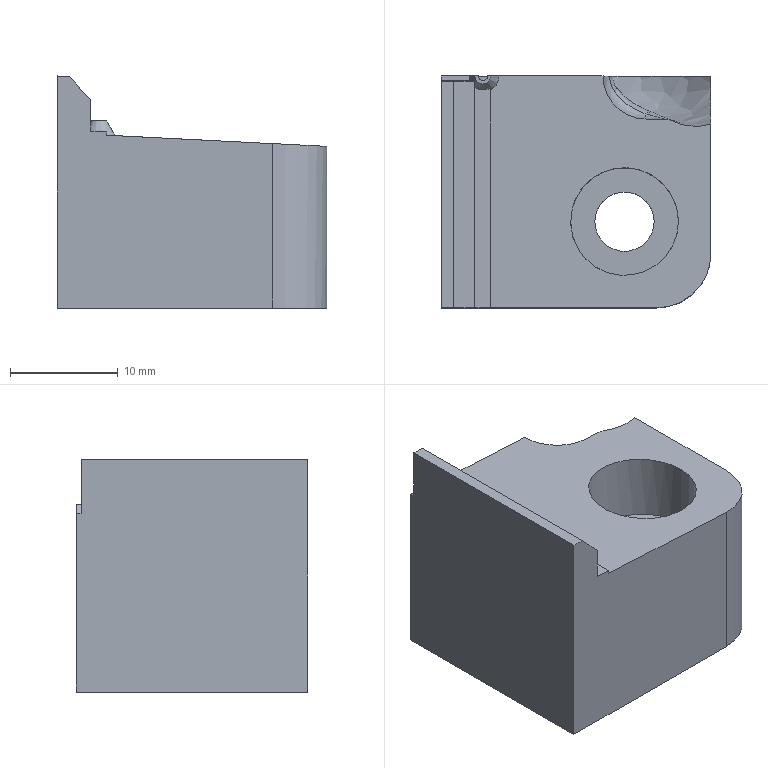Part | STEP file | solid 198 | 1 solid | 31 faces | box 25 x 21.5 x 21.524 mm | volume 7423 mm3 | plane 15 | spline 9 | cylinder 5 | cone 1 | sphere 1 | commonest cylinder face diameters 10 x2 5.5 x1 8 x1 6922 x1